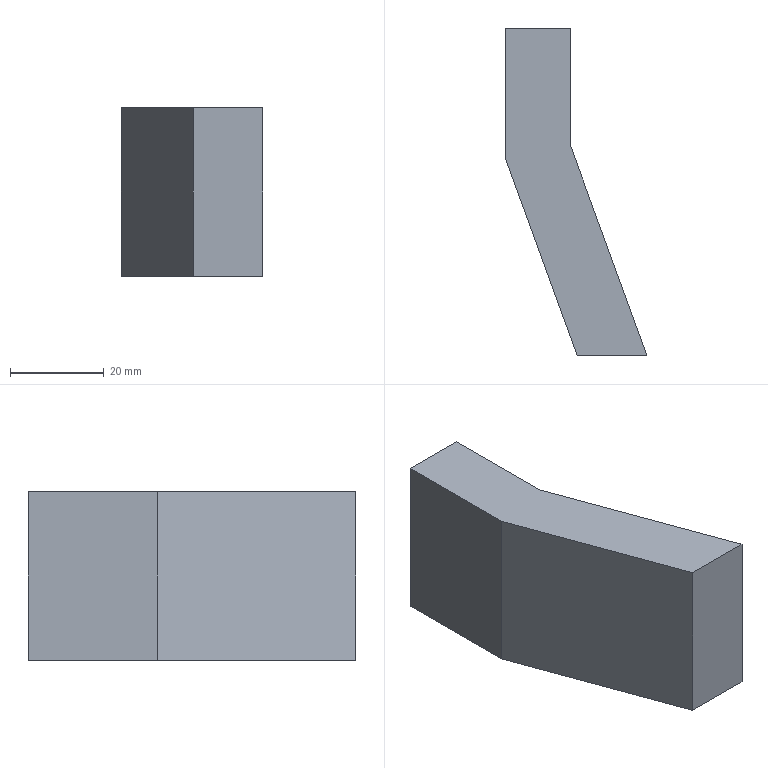Part | NX | features solid 2 | 1 solid | 8 faces | box 30.314 x 70 x 36 mm | volume 36690 mm3 | plane 8
STEP:
#1=CARTESIAN_POINT('',(300.,150.,9.));
#2=VERTEX_POINT('',#1);
#3=CARTESIAN_POINT('',(300.,122.355,9.));
#4=VERTEX_POINT('',#3);
#5=CARTESIAN_POINT('',(300.,150.,9.));
#6=DIRECTION('',(0.,-1.,0.));
#7=VECTOR('',#6,1000.);
#8=LINE('',#5,#7);
#9=EDGE_CURVE('',#2,#4,#8,.T.);
#10=ORIENTED_EDGE('',*,*,#9,.T.);
#11=CARTESIAN_POINT('',(300.,122.355,45.));
#12=VERTEX_POINT('',#11);
#13=CARTESIAN_POINT('',(300.,122.355,45.));
#14=DIRECTION('',(0.,0.,-1.));
#15=VECTOR('',#14,1000.);
#16=LINE('',#13,#15);
#17=EDGE_CURVE('',#12,#4,#16,.T.);
#18=ORIENTED_EDGE('',*,*,#17,.F.);
#19=CARTESIAN_POINT('',(300.,150.,45.));
#20=VERTEX_POINT('',#19);
#21=CARTESIAN_POINT('',(300.,150.,45.));
#22=DIRECTION('',(0.,-1.,0.));
#23=VECTOR('',#22,1000.);
#24=LINE('',#21,#23);
#25=EDGE_CURVE('',#20,#12,#24,.T.);
#26=ORIENTED_EDGE('',*,*,#25,.F.);
#27=CARTESIAN_POINT('',(300.,150.,45.));
#28=DIRECTION('',(0.,0.,-1.));
#29=VECTOR('',#28,1000.);
#30=LINE('',#27,#29);
#31=EDGE_CURVE('',#20,#2,#30,.T.);
#32=ORIENTED_EDGE('',*,*,#31,.T.);
#33=EDGE_LOOP('',(#10,#18,#26,#32));
#34=FACE_BOUND('',#33,.T.);
#35=CARTESIAN_POINT('',(300.,150.,45.));
#36=DIRECTION('',(1.,0.,0.));
#37=DIRECTION('',(0.,1.,0.));
#38=AXIS2_PLACEMENT_3D('',#35,#36,#37);
#39=PLANE('',#38);
#40=ADVANCED_FACE('',(#34),#39,.F.);
#41=CARTESIAN_POINT('',(315.416,80.,9.));
#42=VERTEX_POINT('',#41);
#43=CARTESIAN_POINT('',(300.,122.355,9.));
#44=DIRECTION('',(0.342,-0.9397,0.));
#45=VECTOR('',#44,1000.);
#46=LINE('',#43,#45);
#47=EDGE_CURVE('',#4,#42,#46,.T.);
#48=ORIENTED_EDGE('',*,*,#47,.T.);
#49=CARTESIAN_POINT('',(315.416,80.,45.));
#50=VERTEX_POINT('',#49);
#51=CARTESIAN_POINT('',(315.416,80.,45.));
#52=DIRECTION('',(0.,0.,-1.));
#53=VECTOR('',#52,1000.);
#54=LINE('',#51,#53);
#55=EDGE_CURVE('',#50,#42,#54,.T.);
#56=ORIENTED_EDGE('',*,*,#55,.F.);
#57=CARTESIAN_POINT('',(300.,122.355,45.));
#58=DIRECTION('',(0.342,-0.9397,0.));
#59=VECTOR('',#58,1000.);
#60=LINE('',#57,#59);
#61=EDGE_CURVE('',#12,#50,#60,.T.);
#62=ORIENTED_EDGE('',*,*,#61,.F.);
#63=ORIENTED_EDGE('',*,*,#17,.T.);
#64=EDGE_LOOP('',(#48,#56,#62,#63));
#65=FACE_BOUND('',#64,.T.);
#66=CARTESIAN_POINT('',(300.,122.355,45.));
#67=DIRECTION('',(0.9397,0.342,0.));
#68=DIRECTION('',(-0.342,0.9397,0.));
#69=AXIS2_PLACEMENT_3D('',#66,#67,#68);
#70=PLANE('',#69);
#71=ADVANCED_FACE('',(#65),#70,.F.);
#72=CARTESIAN_POINT('',(330.314,80.,9.));
#73=VERTEX_POINT('',#72);
#74=CARTESIAN_POINT('',(330.314,80.,9.));
#75=DIRECTION('',(-1.,0.,0.));
#76=VECTOR('',#75,1000.);
#77=LINE('',#74,#76);
#78=EDGE_CURVE('',#73,#42,#77,.T.);
#79=ORIENTED_EDGE('',*,*,#78,.F.);
#80=CARTESIAN_POINT('',(330.314,80.,45.));
#81=VERTEX_POINT('',#80);
#82=CARTESIAN_POINT('',(330.314,80.,45.));
#83=DIRECTION('',(0.,0.,-1.));
#84=VECTOR('',#83,1000.);
#85=LINE('',#82,#84);
#86=EDGE_CURVE('',#81,#73,#85,.T.);
#87=ORIENTED_EDGE('',*,*,#86,.F.);
#88=CARTESIAN_POINT('',(330.314,80.,45.));
#89=DIRECTION('',(-1.,0.,0.));
#90=VECTOR('',#89,1000.);
#91=LINE('',#88,#90);
#92=EDGE_CURVE('',#81,#50,#91,.T.);
#93=ORIENTED_EDGE('',*,*,#92,.T.);
#94=ORIENTED_EDGE('',*,*,#55,.T.);
#95=EDGE_LOOP('',(#79,#87,#93,#94));
#96=FACE_BOUND('',#95,.T.);
#97=CARTESIAN_POINT('',(330.314,80.,45.));
#98=DIRECTION('',(0.,-1.,0.));
#99=DIRECTION('',(0.,0.,-1.));
#100=AXIS2_PLACEMENT_3D('',#97,#98,#99);
#101=PLANE('',#100);
#102=ADVANCED_FACE('',(#96),#101,.T.);
#103=CARTESIAN_POINT('',(314.,124.824,9.));
#104=VERTEX_POINT('',#103);
#105=CARTESIAN_POINT('',(314.,124.824,9.));
#106=DIRECTION('',(0.342,-0.9397,0.));
#107=VECTOR('',#106,1000.);
#108=LINE('',#105,#107);
#109=EDGE_CURVE('',#104,#73,#108,.T.);
#110=ORIENTED_EDGE('',*,*,#109,.F.);
#111=CARTESIAN_POINT('',(314.,124.824,45.));
#112=VERTEX_POINT('',#111);
#113=CARTESIAN_POINT('',(314.,124.824,45.));
#114=DIRECTION('',(0.,0.,-1.));
#115=VECTOR('',#114,1000.);
#116=LINE('',#113,#115);
#117=EDGE_CURVE('',#112,#104,#116,.T.);
#118=ORIENTED_EDGE('',*,*,#117,.F.);
#119=CARTESIAN_POINT('',(314.,124.824,45.));
#120=DIRECTION('',(0.342,-0.9397,0.));
#121=VECTOR('',#120,1000.);
#122=LINE('',#119,#121);
#123=EDGE_CURVE('',#112,#81,#122,.T.);
#124=ORIENTED_EDGE('',*,*,#123,.T.);
#125=ORIENTED_EDGE('',*,*,#86,.T.);
#126=EDGE_LOOP('',(#110,#118,#124,#125));
#127=FACE_BOUND('',#126,.T.);
#128=CARTESIAN_POINT('',(314.,124.824,45.));
#129=DIRECTION('',(0.9397,0.342,0.));
#130=DIRECTION('',(-0.342,0.9397,0.));
#131=AXIS2_PLACEMENT_3D('',#128,#129,#130);
#132=PLANE('',#131);
#133=ADVANCED_FACE('',(#127),#132,.T.);
#134=CARTESIAN_POINT('',(314.,150.,9.));
#135=VERTEX_POINT('',#134);
#136=CARTESIAN_POINT('',(314.,150.,9.));
#137=DIRECTION('',(0.,-1.,0.));
#138=VECTOR('',#137,1000.);
#139=LINE('',#136,#138);
#140=EDGE_CURVE('',#135,#104,#139,.T.);
#141=ORIENTED_EDGE('',*,*,#140,.F.);
#142=CARTESIAN_POINT('',(314.,150.,45.));
#143=VERTEX_POINT('',#142);
#144=CARTESIAN_POINT('',(314.,150.,45.));
#145=DIRECTION('',(0.,0.,-1.));
#146=VECTOR('',#145,1000.);
#147=LINE('',#144,#146);
#148=EDGE_CURVE('',#143,#135,#147,.T.);
#149=ORIENTED_EDGE('',*,*,#148,.F.);
#150=CARTESIAN_POINT('',(314.,150.,45.));
#151=DIRECTION('',(0.,-1.,0.));
#152=VECTOR('',#151,1000.);
#153=LINE('',#150,#152);
#154=EDGE_CURVE('',#143,#112,#153,.T.);
#155=ORIENTED_EDGE('',*,*,#154,.T.);
#156=ORIENTED_EDGE('',*,*,#117,.T.);
#157=EDGE_LOOP('',(#141,#149,#155,#156));
#158=FACE_BOUND('',#157,.T.);
#159=CARTESIAN_POINT('',(314.,150.,45.));
#160=DIRECTION('',(1.,0.,0.));
#161=DIRECTION('',(0.,0.,-1.));
#162=AXIS2_PLACEMENT_3D('',#159,#160,#161);
#163=PLANE('',#162);
#164=ADVANCED_FACE('',(#158),#163,.T.);
#165=CARTESIAN_POINT('',(314.,150.,9.));
#166=DIRECTION('',(-1.,0.,0.));
#167=VECTOR('',#166,1000.);
#168=LINE('',#165,#167);
#169=EDGE_CURVE('',#135,#2,#168,.T.);
#170=ORIENTED_EDGE('',*,*,#169,.T.);
#171=ORIENTED_EDGE('',*,*,#31,.F.);
#172=CARTESIAN_POINT('',(314.,150.,45.));
#173=DIRECTION('',(-1.,0.,0.));
#174=VECTOR('',#173,1000.);
#175=LINE('',#172,#174);
#176=EDGE_CURVE('',#143,#20,#175,.T.);
#177=ORIENTED_EDGE('',*,*,#176,.F.);
#178=ORIENTED_EDGE('',*,*,#148,.T.);
#179=EDGE_LOOP('',(#170,#171,#177,#178));
#180=FACE_BOUND('',#179,.T.);
#181=CARTESIAN_POINT('',(314.,150.,45.));
#182=DIRECTION('',(0.,-1.,0.));
#183=DIRECTION('',(0.,0.,-1.));
#184=AXIS2_PLACEMENT_3D('',#181,#182,#183);
#185=PLANE('',#184);
#186=ADVANCED_FACE('',(#180),#185,.F.);
#187=ORIENTED_EDGE('',*,*,#25,.T.);
#188=ORIENTED_EDGE('',*,*,#61,.T.);
#189=ORIENTED_EDGE('',*,*,#92,.F.);
#190=ORIENTED_EDGE('',*,*,#123,.F.);
#191=ORIENTED_EDGE('',*,*,#154,.F.);
#192=ORIENTED_EDGE('',*,*,#176,.T.);
#193=EDGE_LOOP('',(#187,#188,#189,#190,#191,#192));
#194=FACE_BOUND('',#193,.T.);
#195=CARTESIAN_POINT('',(312.288,117.863,45.));
#196=DIRECTION('',(0.,0.,1.));
#197=DIRECTION('',(1.,0.,0.));
#198=AXIS2_PLACEMENT_3D('',#195,#196,#197);
#199=PLANE('',#198);
#200=ADVANCED_FACE('',(#194),#199,.T.);
#201=ORIENTED_EDGE('',*,*,#9,.F.);
#202=ORIENTED_EDGE('',*,*,#169,.F.);
#203=ORIENTED_EDGE('',*,*,#140,.T.);
#204=ORIENTED_EDGE('',*,*,#109,.T.);
#205=ORIENTED_EDGE('',*,*,#78,.T.);
#206=ORIENTED_EDGE('',*,*,#47,.F.);
#207=EDGE_LOOP('',(#201,#202,#203,#204,#205,#206));
#208=FACE_BOUND('',#207,.T.);
#209=CARTESIAN_POINT('',(312.288,117.863,9.));
#210=DIRECTION('',(0.,0.,1.));
#211=DIRECTION('',(1.,0.,0.));
#212=AXIS2_PLACEMENT_3D('',#209,#210,#211);
#213=PLANE('',#212);
#214=ADVANCED_FACE('',(#208),#213,.F.);
#215=CLOSED_SHELL('',(#40,#71,#102,#133,#164,#186,#200,#214));
#216=MANIFOLD_SOLID_BREP('',#215);
#217=(LENGTH_UNIT()NAMED_UNIT(*)SI_UNIT(.MILLI.,.METRE.));
#218=UNCERTAINTY_MEASURE_WITH_UNIT(LENGTH_MEASURE(0.00001),#217,'','');
#219=(NAMED_UNIT(*)PLANE_ANGLE_UNIT()SI_UNIT($,.RADIAN.));
#220=(NAMED_UNIT(*)SI_UNIT($,.STERADIAN.)SOLID_ANGLE_UNIT());
#221=(GEOMETRIC_REPRESENTATION_CONTEXT(3)GLOBAL_UNCERTAINTY_ASSIGNED_CONTEXT((#218))GLOBAL_UNIT_ASSIGNED_CONTEXT((#217,#219,#220))REPRESENTATION_CONTEXT('',''));
#222=ADVANCED_BREP_SHAPE_REPRESENTATION('',(#216),#221);